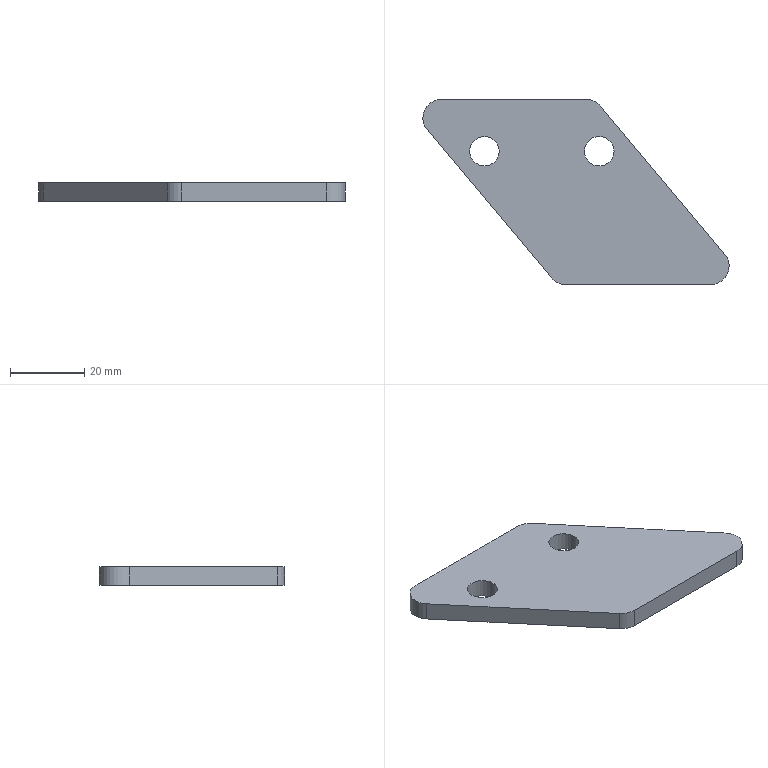Part | STEP file | 6151204 | 1 solid | 12 faces | box 82.726 x 50 x 5 mm | volume 12291 mm3 | plane 6 | cylinder 6 | commonest cylinder face diameters 10 x4 8 x2
STEP:
#1=CARTESIAN_POINT('',(2.799,25.,5.));
#2=VERTEX_POINT('',#1);
#3=CARTESIAN_POINT('',(-36.363,25.,5.));
#4=VERTEX_POINT('',#3);
#5=CARTESIAN_POINT('',(5.131,25.,5.));
#6=DIRECTION('',(-1.,0.,0.));
#7=VECTOR('',#6,1000.);
#8=LINE('',#5,#7);
#9=EDGE_CURVE('',#2,#4,#8,.T.);
#10=ORIENTED_EDGE('',*,*,#9,.F.);
#11=CARTESIAN_POINT('',(2.799,25.,0.));
#12=VERTEX_POINT('',#11);
#13=CARTESIAN_POINT('',(2.799,25.,5.));
#14=DIRECTION('',(0.,0.,-1.));
#15=VECTOR('',#14,1000.);
#16=LINE('',#13,#15);
#17=EDGE_CURVE('',#2,#12,#16,.T.);
#18=ORIENTED_EDGE('',*,*,#17,.T.);
#19=CARTESIAN_POINT('',(-36.363,25.,0.));
#20=VERTEX_POINT('',#19);
#21=CARTESIAN_POINT('',(5.131,25.,0.));
#22=DIRECTION('',(-1.,0.,0.));
#23=VECTOR('',#22,1000.);
#24=LINE('',#21,#23);
#25=EDGE_CURVE('',#12,#20,#24,.T.);
#26=ORIENTED_EDGE('',*,*,#25,.T.);
#27=CARTESIAN_POINT('',(-36.363,25.,5.));
#28=DIRECTION('',(0.,0.,1.));
#29=VECTOR('',#28,1000.);
#30=LINE('',#27,#29);
#31=EDGE_CURVE('',#20,#4,#30,.T.);
#32=ORIENTED_EDGE('',*,*,#31,.T.);
#33=EDGE_LOOP('',(#10,#18,#26,#32));
#34=FACE_OUTER_BOUND('',#33,.T.);
#35=CARTESIAN_POINT('',(5.131,25.,5.));
#36=DIRECTION('',(0.,-1.,0.));
#37=DIRECTION('',(1.,0.,0.));
#38=AXIS2_PLACEMENT_3D('',#35,#36,#37);
#39=PLANE('',#38);
#40=ADVANCED_FACE('',(#34),#39,.F.);
#41=CARTESIAN_POINT('',(-40.193,16.786,0.));
#42=VERTEX_POINT('',#41);
#43=CARTESIAN_POINT('',(-6.629,-23.214,0.));
#44=VERTEX_POINT('',#43);
#45=CARTESIAN_POINT('',(-47.086,25.,0.));
#46=DIRECTION('',(0.6428,-0.766,0.));
#47=VECTOR('',#46,1000.);
#48=LINE('',#45,#47);
#49=EDGE_CURVE('',#42,#44,#48,.T.);
#50=ORIENTED_EDGE('',*,*,#49,.T.);
#51=CARTESIAN_POINT('',(-6.629,-23.214,5.));
#52=VERTEX_POINT('',#51);
#53=CARTESIAN_POINT('',(-6.629,-23.214,5.));
#54=DIRECTION('',(0.,0.,1.));
#55=VECTOR('',#54,1000.);
#56=LINE('',#53,#55);
#57=EDGE_CURVE('',#44,#52,#56,.T.);
#58=ORIENTED_EDGE('',*,*,#57,.T.);
#59=CARTESIAN_POINT('',(-40.193,16.786,5.));
#60=VERTEX_POINT('',#59);
#61=CARTESIAN_POINT('',(-47.086,25.,5.));
#62=DIRECTION('',(0.6428,-0.766,0.));
#63=VECTOR('',#62,1000.);
#64=LINE('',#61,#63);
#65=EDGE_CURVE('',#60,#52,#64,.T.);
#66=ORIENTED_EDGE('',*,*,#65,.F.);
#67=CARTESIAN_POINT('',(-40.193,16.786,5.));
#68=DIRECTION('',(0.,0.,-1.));
#69=VECTOR('',#68,1000.);
#70=LINE('',#67,#69);
#71=EDGE_CURVE('',#60,#42,#70,.T.);
#72=ORIENTED_EDGE('',*,*,#71,.T.);
#73=EDGE_LOOP('',(#50,#58,#66,#72));
#74=FACE_OUTER_BOUND('',#73,.T.);
#75=CARTESIAN_POINT('',(-47.086,25.,5.));
#76=DIRECTION('',(0.766,0.6428,0.));
#77=DIRECTION('',(-0.6428,0.766,0.));
#78=AXIS2_PLACEMENT_3D('',#75,#76,#77);
#79=PLANE('',#78);
#80=ADVANCED_FACE('',(#74),#79,.F.);
#81=CARTESIAN_POINT('',(-2.799,-25.,5.));
#82=VERTEX_POINT('',#81);
#83=CARTESIAN_POINT('',(36.363,-25.,5.));
#84=VERTEX_POINT('',#83);
#85=CARTESIAN_POINT('',(-5.131,-25.,5.));
#86=DIRECTION('',(1.,0.,0.));
#87=VECTOR('',#86,1000.);
#88=LINE('',#85,#87);
#89=EDGE_CURVE('',#82,#84,#88,.T.);
#90=ORIENTED_EDGE('',*,*,#89,.F.);
#91=CARTESIAN_POINT('',(-2.799,-25.,0.));
#92=VERTEX_POINT('',#91);
#93=CARTESIAN_POINT('',(-2.799,-25.,5.));
#94=DIRECTION('',(0.,0.,-1.));
#95=VECTOR('',#94,1000.);
#96=LINE('',#93,#95);
#97=EDGE_CURVE('',#82,#92,#96,.T.);
#98=ORIENTED_EDGE('',*,*,#97,.T.);
#99=CARTESIAN_POINT('',(36.363,-25.,0.));
#100=VERTEX_POINT('',#99);
#101=CARTESIAN_POINT('',(-5.131,-25.,0.));
#102=DIRECTION('',(1.,0.,0.));
#103=VECTOR('',#102,1000.);
#104=LINE('',#101,#103);
#105=EDGE_CURVE('',#92,#100,#104,.T.);
#106=ORIENTED_EDGE('',*,*,#105,.T.);
#107=CARTESIAN_POINT('',(36.363,-25.,5.));
#108=DIRECTION('',(0.,0.,1.));
#109=VECTOR('',#108,1000.);
#110=LINE('',#107,#109);
#111=EDGE_CURVE('',#100,#84,#110,.T.);
#112=ORIENTED_EDGE('',*,*,#111,.T.);
#113=EDGE_LOOP('',(#90,#98,#106,#112));
#114=FACE_OUTER_BOUND('',#113,.T.);
#115=CARTESIAN_POINT('',(-5.131,-25.,5.));
#116=DIRECTION('',(0.,1.,0.));
#117=DIRECTION('',(-1.,0.,0.));
#118=AXIS2_PLACEMENT_3D('',#115,#116,#117);
#119=PLANE('',#118);
#120=ADVANCED_FACE('',(#114),#119,.F.);
#121=CARTESIAN_POINT('',(40.193,-16.786,5.));
#122=VERTEX_POINT('',#121);
#123=CARTESIAN_POINT('',(6.629,23.214,5.));
#124=VERTEX_POINT('',#123);
#125=CARTESIAN_POINT('',(47.086,-25.,5.));
#126=DIRECTION('',(-0.6428,0.766,0.));
#127=VECTOR('',#126,1000.);
#128=LINE('',#125,#127);
#129=EDGE_CURVE('',#122,#124,#128,.T.);
#130=ORIENTED_EDGE('',*,*,#129,.F.);
#131=CARTESIAN_POINT('',(40.193,-16.786,0.));
#132=VERTEX_POINT('',#131);
#133=CARTESIAN_POINT('',(40.193,-16.786,5.));
#134=DIRECTION('',(0.,0.,-1.));
#135=VECTOR('',#134,1000.);
#136=LINE('',#133,#135);
#137=EDGE_CURVE('',#122,#132,#136,.T.);
#138=ORIENTED_EDGE('',*,*,#137,.T.);
#139=CARTESIAN_POINT('',(6.629,23.214,0.));
#140=VERTEX_POINT('',#139);
#141=CARTESIAN_POINT('',(47.086,-25.,0.));
#142=DIRECTION('',(-0.6428,0.766,0.));
#143=VECTOR('',#142,1000.);
#144=LINE('',#141,#143);
#145=EDGE_CURVE('',#132,#140,#144,.T.);
#146=ORIENTED_EDGE('',*,*,#145,.T.);
#147=CARTESIAN_POINT('',(6.629,23.214,5.));
#148=DIRECTION('',(0.,0.,1.));
#149=VECTOR('',#148,1000.);
#150=LINE('',#147,#149);
#151=EDGE_CURVE('',#140,#124,#150,.T.);
#152=ORIENTED_EDGE('',*,*,#151,.T.);
#153=EDGE_LOOP('',(#130,#138,#146,#152));
#154=FACE_OUTER_BOUND('',#153,.T.);
#155=CARTESIAN_POINT('',(47.086,-25.,5.));
#156=DIRECTION('',(-0.766,-0.6428,0.));
#157=DIRECTION('',(0.6428,-0.766,0.));
#158=AXIS2_PLACEMENT_3D('',#155,#156,#157);
#159=PLANE('',#158);
#160=ADVANCED_FACE('',(#154),#159,.F.);
#161=CARTESIAN_POINT('',(10.27,11.,5.));
#162=VERTEX_POINT('',#161);
#163=CARTESIAN_POINT('',(6.27,11.,5.));
#164=DIRECTION('',(0.,0.,1.));
#165=DIRECTION('',(1.,0.,0.));
#166=AXIS2_PLACEMENT_3D('',#163,#164,#165);
#167=CIRCLE('',#166,4.);
#168=EDGE_CURVE('',#162,#162,#167,.T.);
#169=ORIENTED_EDGE('',*,*,#168,.F.);
#170=EDGE_LOOP('',(#169));
#171=FACE_BOUND('',#170,.T.);
#172=CARTESIAN_POINT('',(-20.73,11.,5.));
#173=VERTEX_POINT('',#172);
#174=CARTESIAN_POINT('',(-24.73,11.,5.));
#175=DIRECTION('',(0.,0.,1.));
#176=DIRECTION('',(1.,0.,0.));
#177=AXIS2_PLACEMENT_3D('',#174,#175,#176);
#178=CIRCLE('',#177,4.);
#179=EDGE_CURVE('',#173,#173,#178,.T.);
#180=ORIENTED_EDGE('',*,*,#179,.F.);
#181=EDGE_LOOP('',(#180));
#182=FACE_BOUND('',#181,.T.);
#183=ORIENTED_EDGE('',*,*,#65,.T.);
#184=CARTESIAN_POINT('',(-2.799,-20.,5.));
#185=DIRECTION('',(0.,0.,1.));
#186=DIRECTION('',(1.,0.,0.));
#187=AXIS2_PLACEMENT_3D('',#184,#185,#186);
#188=CIRCLE('',#187,5.);
#189=EDGE_CURVE('',#52,#82,#188,.T.);
#190=ORIENTED_EDGE('',*,*,#189,.T.);
#191=ORIENTED_EDGE('',*,*,#89,.T.);
#192=CARTESIAN_POINT('',(36.363,-20.,5.));
#193=DIRECTION('',(0.,0.,1.));
#194=DIRECTION('',(1.,0.,0.));
#195=AXIS2_PLACEMENT_3D('',#192,#193,#194);
#196=CIRCLE('',#195,5.);
#197=EDGE_CURVE('',#84,#122,#196,.T.);
#198=ORIENTED_EDGE('',*,*,#197,.T.);
#199=ORIENTED_EDGE('',*,*,#129,.T.);
#200=CARTESIAN_POINT('',(2.799,20.,5.));
#201=DIRECTION('',(0.,0.,1.));
#202=DIRECTION('',(1.,0.,0.));
#203=AXIS2_PLACEMENT_3D('',#200,#201,#202);
#204=CIRCLE('',#203,5.);
#205=EDGE_CURVE('',#124,#2,#204,.T.);
#206=ORIENTED_EDGE('',*,*,#205,.T.);
#207=ORIENTED_EDGE('',*,*,#9,.T.);
#208=CARTESIAN_POINT('',(-36.363,20.,5.));
#209=DIRECTION('',(0.,0.,1.));
#210=DIRECTION('',(1.,0.,0.));
#211=AXIS2_PLACEMENT_3D('',#208,#209,#210);
#212=CIRCLE('',#211,5.);
#213=EDGE_CURVE('',#4,#60,#212,.T.);
#214=ORIENTED_EDGE('',*,*,#213,.T.);
#215=EDGE_LOOP('',(#183,#190,#191,#198,#199,#206,#207,#214));
#216=FACE_OUTER_BOUND('',#215,.T.);
#217=CARTESIAN_POINT('',(-47.086,25.,5.));
#218=DIRECTION('',(0.,0.,1.));
#219=DIRECTION('',(1.,0.,0.));
#220=AXIS2_PLACEMENT_3D('',#217,#218,#219);
#221=PLANE('',#220);
#222=ADVANCED_FACE('',(#171,#182,#216),#221,.T.);
#223=CARTESIAN_POINT('',(2.27,11.,0.));
#224=VERTEX_POINT('',#223);
#225=CARTESIAN_POINT('',(6.27,11.,0.));
#226=DIRECTION('',(0.,0.,-1.));
#227=DIRECTION('',(-1.,0.,0.));
#228=AXIS2_PLACEMENT_3D('',#225,#226,#227);
#229=CIRCLE('',#228,4.);
#230=EDGE_CURVE('',#224,#224,#229,.T.);
#231=ORIENTED_EDGE('',*,*,#230,.F.);
#232=EDGE_LOOP('',(#231));
#233=FACE_BOUND('',#232,.T.);
#234=CARTESIAN_POINT('',(-28.73,11.,0.));
#235=VERTEX_POINT('',#234);
#236=CARTESIAN_POINT('',(-24.73,11.,0.));
#237=DIRECTION('',(0.,0.,-1.));
#238=DIRECTION('',(-1.,0.,0.));
#239=AXIS2_PLACEMENT_3D('',#236,#237,#238);
#240=CIRCLE('',#239,4.);
#241=EDGE_CURVE('',#235,#235,#240,.T.);
#242=ORIENTED_EDGE('',*,*,#241,.F.);
#243=EDGE_LOOP('',(#242));
#244=FACE_BOUND('',#243,.T.);
#245=ORIENTED_EDGE('',*,*,#105,.F.);
#246=CARTESIAN_POINT('',(-2.799,-20.,0.));
#247=DIRECTION('',(0.,0.,-1.));
#248=DIRECTION('',(1.,0.,0.));
#249=AXIS2_PLACEMENT_3D('',#246,#247,#248);
#250=CIRCLE('',#249,5.);
#251=EDGE_CURVE('',#92,#44,#250,.T.);
#252=ORIENTED_EDGE('',*,*,#251,.T.);
#253=ORIENTED_EDGE('',*,*,#49,.F.);
#254=CARTESIAN_POINT('',(-36.363,20.,0.));
#255=DIRECTION('',(0.,0.,-1.));
#256=DIRECTION('',(1.,0.,0.));
#257=AXIS2_PLACEMENT_3D('',#254,#255,#256);
#258=CIRCLE('',#257,5.);
#259=EDGE_CURVE('',#42,#20,#258,.T.);
#260=ORIENTED_EDGE('',*,*,#259,.T.);
#261=ORIENTED_EDGE('',*,*,#25,.F.);
#262=CARTESIAN_POINT('',(2.799,20.,0.));
#263=DIRECTION('',(0.,0.,-1.));
#264=DIRECTION('',(1.,0.,0.));
#265=AXIS2_PLACEMENT_3D('',#262,#263,#264);
#266=CIRCLE('',#265,5.);
#267=EDGE_CURVE('',#12,#140,#266,.T.);
#268=ORIENTED_EDGE('',*,*,#267,.T.);
#269=ORIENTED_EDGE('',*,*,#145,.F.);
#270=CARTESIAN_POINT('',(36.363,-20.,0.));
#271=DIRECTION('',(0.,0.,-1.));
#272=DIRECTION('',(1.,0.,0.));
#273=AXIS2_PLACEMENT_3D('',#270,#271,#272);
#274=CIRCLE('',#273,5.);
#275=EDGE_CURVE('',#132,#100,#274,.T.);
#276=ORIENTED_EDGE('',*,*,#275,.T.);
#277=EDGE_LOOP('',(#245,#252,#253,#260,#261,#268,#269,#276));
#278=FACE_OUTER_BOUND('',#277,.T.);
#279=CARTESIAN_POINT('',(-47.086,25.,0.));
#280=DIRECTION('',(0.,0.,1.));
#281=DIRECTION('',(1.,0.,0.));
#282=AXIS2_PLACEMENT_3D('',#279,#280,#281);
#283=PLANE('',#282);
#284=ADVANCED_FACE('',(#233,#244,#278),#283,.F.);
#285=ORIENTED_EDGE('',*,*,#189,.F.);
#286=ORIENTED_EDGE('',*,*,#57,.F.);
#287=ORIENTED_EDGE('',*,*,#251,.F.);
#288=ORIENTED_EDGE('',*,*,#97,.F.);
#289=EDGE_LOOP('',(#285,#286,#287,#288));
#290=FACE_OUTER_BOUND('',#289,.T.);
#291=CARTESIAN_POINT('',(-2.799,-20.,5.));
#292=DIRECTION('',(0.,0.,-1.));
#293=DIRECTION('',(-1.,0.,0.));
#294=AXIS2_PLACEMENT_3D('',#291,#292,#293);
#295=CYLINDRICAL_SURFACE('',#294,5.);
#296=ADVANCED_FACE('',(#290),#295,.T.);
#297=ORIENTED_EDGE('',*,*,#197,.F.);
#298=ORIENTED_EDGE('',*,*,#111,.F.);
#299=ORIENTED_EDGE('',*,*,#275,.F.);
#300=ORIENTED_EDGE('',*,*,#137,.F.);
#301=EDGE_LOOP('',(#297,#298,#299,#300));
#302=FACE_OUTER_BOUND('',#301,.T.);
#303=CARTESIAN_POINT('',(36.363,-20.,5.));
#304=DIRECTION('',(0.,0.,-1.));
#305=DIRECTION('',(-1.,0.,0.));
#306=AXIS2_PLACEMENT_3D('',#303,#304,#305);
#307=CYLINDRICAL_SURFACE('',#306,5.);
#308=ADVANCED_FACE('',(#302),#307,.T.);
#309=ORIENTED_EDGE('',*,*,#205,.F.);
#310=ORIENTED_EDGE('',*,*,#151,.F.);
#311=ORIENTED_EDGE('',*,*,#267,.F.);
#312=ORIENTED_EDGE('',*,*,#17,.F.);
#313=EDGE_LOOP('',(#309,#310,#311,#312));
#314=FACE_OUTER_BOUND('',#313,.T.);
#315=CARTESIAN_POINT('',(2.799,20.,5.));
#316=DIRECTION('',(0.,0.,-1.));
#317=DIRECTION('',(-1.,0.,0.));
#318=AXIS2_PLACEMENT_3D('',#315,#316,#317);
#319=CYLINDRICAL_SURFACE('',#318,5.);
#320=ADVANCED_FACE('',(#314),#319,.T.);
#321=ORIENTED_EDGE('',*,*,#213,.F.);
#322=ORIENTED_EDGE('',*,*,#31,.F.);
#323=ORIENTED_EDGE('',*,*,#259,.F.);
#324=ORIENTED_EDGE('',*,*,#71,.F.);
#325=EDGE_LOOP('',(#321,#322,#323,#324));
#326=FACE_OUTER_BOUND('',#325,.T.);
#327=CARTESIAN_POINT('',(-36.363,20.,5.));
#328=DIRECTION('',(0.,0.,-1.));
#329=DIRECTION('',(-1.,0.,0.));
#330=AXIS2_PLACEMENT_3D('',#327,#328,#329);
#331=CYLINDRICAL_SURFACE('',#330,5.);
#332=ADVANCED_FACE('',(#326),#331,.T.);
#333=ORIENTED_EDGE('',*,*,#179,.T.);
#334=EDGE_LOOP('',(#333));
#335=FACE_OUTER_BOUND('',#334,.T.);
#336=ORIENTED_EDGE('',*,*,#241,.T.);
#337=EDGE_LOOP('',(#336));
#338=FACE_OUTER_BOUND('',#337,.T.);
#339=CARTESIAN_POINT('',(-24.73,11.,10.));
#340=DIRECTION('',(0.,0.,-1.));
#341=DIRECTION('',(-1.,0.,0.));
#342=AXIS2_PLACEMENT_3D('',#339,#340,#341);
#343=CYLINDRICAL_SURFACE('',#342,4.);
#344=ADVANCED_FACE('',(#335,#338),#343,.F.);
#345=ORIENTED_EDGE('',*,*,#168,.T.);
#346=EDGE_LOOP('',(#345));
#347=FACE_OUTER_BOUND('',#346,.T.);
#348=ORIENTED_EDGE('',*,*,#230,.T.);
#349=EDGE_LOOP('',(#348));
#350=FACE_OUTER_BOUND('',#349,.T.);
#351=CARTESIAN_POINT('',(6.27,11.,10.));
#352=DIRECTION('',(0.,0.,-1.));
#353=DIRECTION('',(-1.,0.,0.));
#354=AXIS2_PLACEMENT_3D('',#351,#352,#353);
#355=CYLINDRICAL_SURFACE('',#354,4.);
#356=ADVANCED_FACE('',(#347,#350),#355,.F.);
#357=CLOSED_SHELL('',(#40,#80,#120,#160,#222,#284,#296,#308,#320,#332,#344,#356));
#358=MANIFOLD_SOLID_BREP('',#357);
#359=CARTESIAN_POINT('',(0.,0.,0.));
#360=DIRECTION('',(0.,0.,1.));
#361=DIRECTION('',(1.,0.,0.));
#362=AXIS2_PLACEMENT_3D('',#359,#360,#361);
#363=(LENGTH_UNIT()NAMED_UNIT(*)SI_UNIT(.MILLI.,.METRE.));
#364=UNCERTAINTY_MEASURE_WITH_UNIT(LENGTH_MEASURE(0.00001),#363,'','');
#365=(NAMED_UNIT(*)PLANE_ANGLE_UNIT()SI_UNIT($,.RADIAN.));
#366=(NAMED_UNIT(*)SI_UNIT($,.STERADIAN.)SOLID_ANGLE_UNIT());
#367=(GEOMETRIC_REPRESENTATION_CONTEXT(3)GLOBAL_UNCERTAINTY_ASSIGNED_CONTEXT((#364))GLOBAL_UNIT_ASSIGNED_CONTEXT((#363,#365,#366))REPRESENTATION_CONTEXT('',''));
#368=ADVANCED_BREP_SHAPE_REPRESENTATION('',(#358,#362),#367);